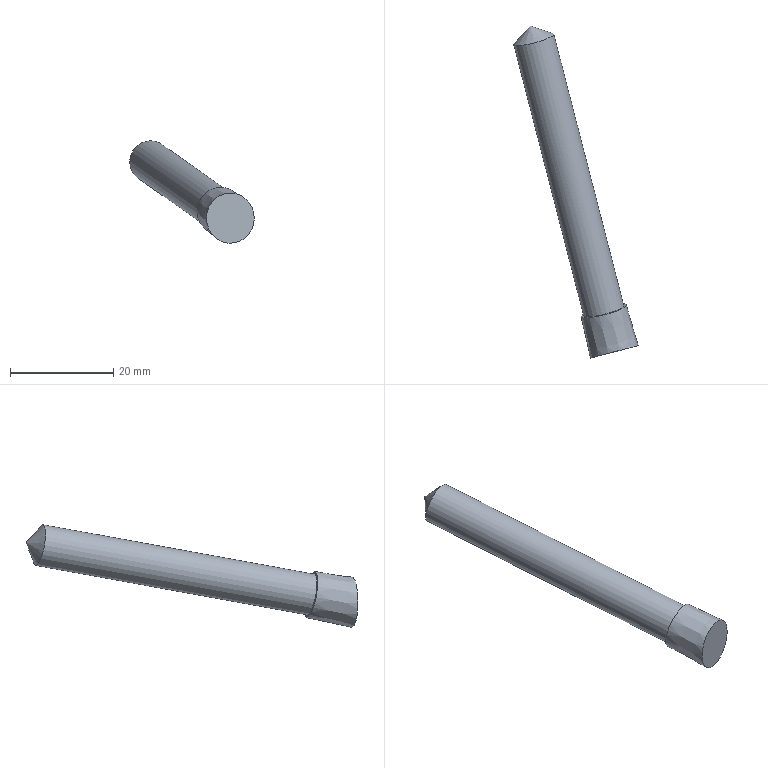Part | STEP file | 车灯-后视镜_id686_x_t | 1 solid | 5 faces | box 24.107 x 64.242 x 19.839 mm | volume 3383 mm3 | plane 2 | cone 2 | cylinder 1 | commonest cylinder face diameters 8 x1
STEP:
#1=CARTESIAN_POINT('',(-8.025,37.639,41.832));
#2=VERTEX_POINT('',#1);
#3=CARTESIAN_POINT('',(-4.152,38.638,41.832));
#4=DIRECTION('',(0.2459,-0.9536,-0.1736));
#5=DIRECTION('',(-0.9683,-0.2497,0.));
#6=AXIS2_PLACEMENT_3D('',#3,#4,#5);
#7=CIRCLE('',#6,4.);
#8=EDGE_CURVE('',#2,#2,#7,.T.);
#9=ORIENTED_EDGE('',*,*,#8,.T.);
#10=EDGE_LOOP('',(#9));
#11=FACE_BOUND('',#10,.T.);
#12=CARTESIAN_POINT('',(-4.348,39.401,37.366));
#13=VERTEX_POINT('',#12);
#14=CARTESIAN_POINT('',(-4.152,38.638,41.832));
#15=DIRECTION('',(-0.2459,0.9536,0.1736));
#16=DIRECTION('',(-0.04336,0.1681,-0.9848));
#17=AXIS2_PLACEMENT_3D('',#14,#15,#16);
#18=CIRCLE('',#17,4.535);
#19=EDGE_CURVE('',#13,#13,#18,.T.);
#20=ORIENTED_EDGE('',*,*,#19,.T.);
#21=EDGE_LOOP('',(#20));
#22=FACE_BOUND('',#21,.T.);
#23=CARTESIAN_POINT('',(-4.152,38.638,41.832));
#24=DIRECTION('',(-0.2459,0.9536,0.1736));
#25=DIRECTION('',(0.04336,-0.1681,0.9848));
#26=AXIS2_PLACEMENT_3D('',#23,#24,#25);
#27=PLANE('',#26);
#28=ADVANCED_FACE('',(#11,#22),#27,.T.);
#29=CARTESIAN_POINT('',(-2.104,30.689,35.497));
#30=VERTEX_POINT('',#29);
#31=CARTESIAN_POINT('',(-2.102,30.69,40.359));
#32=DIRECTION('',(0.2498,-0.9683,0.));
#33=DIRECTION('',(-0.0003877,-0.0001,-1.));
#34=AXIS2_PLACEMENT_3D('',#31,#32,#33);
#35=ELLIPSE('',#34,4.862,4.788);
#36=EDGE_CURVE('',#30,#30,#35,.T.);
#37=ORIENTED_EDGE('',*,*,#36,.F.);
#38=EDGE_LOOP('',(#37));
#39=FACE_BOUND('',#38,.T.);
#40=ORIENTED_EDGE('',*,*,#19,.F.);
#41=EDGE_LOOP('',(#40));
#42=FACE_BOUND('',#41,.T.);
#43=CARTESIAN_POINT('',(-4.152,38.638,41.832));
#44=DIRECTION('',(0.2459,-0.9536,-0.1736));
#45=DIRECTION('',(-0.04336,0.1681,-0.9848));
#46=AXIS2_PLACEMENT_3D('',#43,#44,#45);
#47=CONICAL_SURFACE('',#46,4.535,1.738);
#48=ADVANCED_FACE('',(#39,#42),#47,.T.);
#49=ORIENTED_EDGE('',*,*,#8,.F.);
#50=EDGE_LOOP('',(#49));
#51=FACE_BOUND('',#50,.T.);
#52=CARTESIAN_POINT('',(-13.823,92.162,51.397));
#53=VERTEX_POINT('',#52);
#54=CARTESIAN_POINT('',(-17.696,91.163,51.397));
#55=DIRECTION('',(-0.2459,0.9536,0.1736));
#56=DIRECTION('',(0.9683,0.2497,0.));
#57=AXIS2_PLACEMENT_3D('',#54,#55,#56);
#58=CIRCLE('',#57,4.);
#59=EDGE_CURVE('',#53,#53,#58,.T.);
#60=ORIENTED_EDGE('',*,*,#59,.F.);
#61=EDGE_LOOP('',(#60));
#62=FACE_BOUND('',#61,.T.);
#63=CARTESIAN_POINT('',(15.993,-39.482,27.607));
#64=DIRECTION('',(-0.2459,0.9536,0.1736));
#65=DIRECTION('',(0.04336,-0.1681,0.9848));
#66=AXIS2_PLACEMENT_3D('',#63,#64,#65);
#67=CYLINDRICAL_SURFACE('',#66,4.);
#68=ADVANCED_FACE('',(#51,#62),#67,.T.);
#69=ORIENTED_EDGE('',*,*,#59,.T.);
#70=EDGE_LOOP('',(#69));
#71=FACE_BOUND('',#70,.T.);
#72=CARTESIAN_POINT('',(-18.36,93.736,51.865));
#73=VERTEX_POINT('',#72);
#74=VERTEX_LOOP('',#73);
#75=FACE_BOUND('',#74,.T.);
#76=CARTESIAN_POINT('',(-18.36,93.736,51.865));
#77=DIRECTION('',(0.2459,-0.9536,-0.1736));
#78=DIRECTION('',(0.04336,-0.1681,0.9848));
#79=AXIS2_PLACEMENT_3D('',#76,#77,#78);
#80=CONICAL_SURFACE('',#79,0.,56.);
#81=ADVANCED_FACE('',(#71,#75),#80,.T.);
#82=ORIENTED_EDGE('',*,*,#36,.T.);
#83=EDGE_LOOP('',(#82));
#84=FACE_OUTER_BOUND('',#83,.T.);
#85=CARTESIAN_POINT('',(-10.125,28.621,33.596));
#86=DIRECTION('',(-0.2498,0.9683,0.));
#87=DIRECTION('',(-0.9683,-0.2498,0.));
#88=AXIS2_PLACEMENT_3D('',#85,#86,#87);
#89=PLANE('',#88);
#90=ADVANCED_FACE('',(#84),#89,.F.);
#91=CLOSED_SHELL('',(#28,#48,#68,#81,#90));
#92=MANIFOLD_SOLID_BREP('',#91);
#93=(LENGTH_UNIT()NAMED_UNIT(*)SI_UNIT(.MILLI.,.METRE.));
#94=UNCERTAINTY_MEASURE_WITH_UNIT(LENGTH_MEASURE(0.00002),#93,'','');
#95=(NAMED_UNIT(*)PLANE_ANGLE_UNIT()SI_UNIT($,.RADIAN.));
#96=PLANE_ANGLE_MEASURE_WITH_UNIT(PLANE_ANGLE_MEASURE(0.01745),#95);
#97=DIMENSIONAL_EXPONENTS(0.,0.,0.,0.,0.,0.,0.);
#98=(CONVERSION_BASED_UNIT('DEGREE',#96)NAMED_UNIT(#97)PLANE_ANGLE_UNIT());
#99=(NAMED_UNIT(*)SI_UNIT($,.STERADIAN.)SOLID_ANGLE_UNIT());
#100=(GEOMETRIC_REPRESENTATION_CONTEXT(3)GLOBAL_UNCERTAINTY_ASSIGNED_CONTEXT((#94))GLOBAL_UNIT_ASSIGNED_CONTEXT((#93,#98,#99))REPRESENTATION_CONTEXT('',''));
#101=ADVANCED_BREP_SHAPE_REPRESENTATION('',(#92),#100);